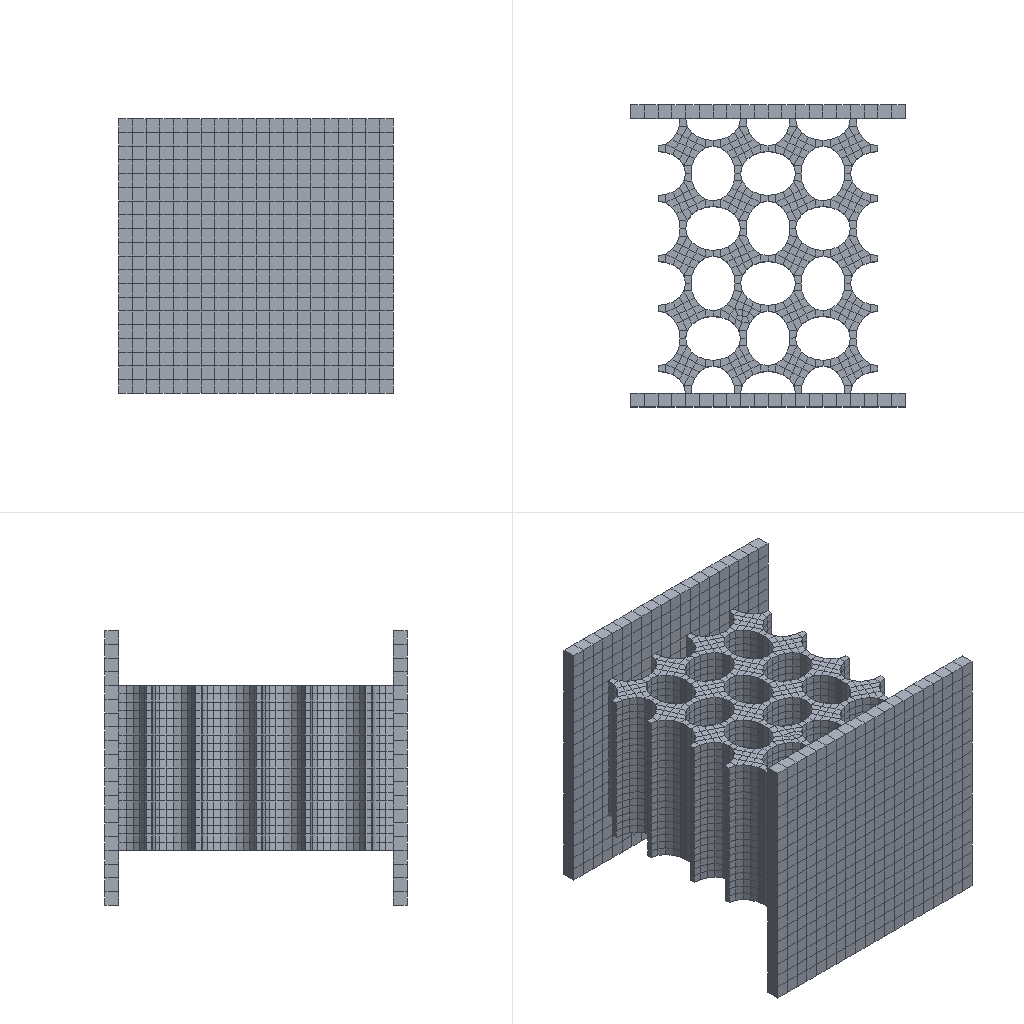Simulation study | abaqus
Set-up summary:
category,name,step,type,value,unit,region
solver,abaqus,,Abaqus/CAE 2024
units,mm-N-s-tonne (MPa),,inferred,E=210000 density=7.89e-09
analysis,Step-1,,dynamic explicit,nlgeom=True; time_period=0.1
mesh,nodes,,,14387
mesh,elements,,,8860
element_type,C3D8R,,,8860
material,Steel,,E,210000
material,Steel,,nu,0.3
material,Steel,,density,7.89e-09
material,TPU,,E,450
material,TPU,,nu,0.38
material,TPU,,density,1.25e-09
material,TPU,,yield,28
material,TPU,,behaviors,plastic
section,Steel,,solid section,,,Bottom
section,Steel,,solid section,,,Head
section,TPU,,solid section,,,JG
bc,BC-1,initial,encastre,[dofs=ENCASTRE],,_PickedSet27
bc,BC-2,Step-1,fixed,"[dofs=rx,ry,rz,x,z n=5]",,_PickedSet28
bc,BC-2,Step-1,displacement,-10 [dofs=y],,_PickedSet28
contact,Int-1,initial,general contact,interaction=IntProp-1; friction=0.2; behavior=hard
constraint,rigid body,,,2
Abaqus input file, long lists of numbers shortened:
*Heading
** Job name: deck Model name: 0204
** Generated by: Abaqus/CAE 2024
*Preprint, echo=NO, model=NO, history=NO, contact=NO
**
** PARTS
**
*Part, name=Bottom
*Node
      1,          20.,          20.,           1.
      2,          20.,          19.,           1.
** (880 more lines like these left out)
*Element, type=C3D8R
  1,  43,  44,  65,  64,   1,   2,  23,  22
  2,  44,  45,  66,  65,   2,   3,  24,  23
** (398 more lines like these left out)
*Nset, nset=Bottom, generate
   1,  882,    1
*Elset, elset=Bottom, generate
   1,  400,    1
** Section: YABAN
*Solid Section, elset=Bottom, material=Steel
,
*End Part
**
*Part, name=Head
*Node
      1,          20.,          20.,           1.
      2,          20.,          19.,           1.
** (880 more lines like these left out)
*Element, type=C3D8R
  1,  43,  44,  65,  64,   1,   2,  23,  22
  2,  44,  45,  66,  65,   2,   3,  24,  23
** (398 more lines like these left out)
*Nset, nset=Head, generate
   1,  882,    1
*Elset, elset=Head, generate
   1,  400,    1
** Section: YABAN
*Solid Section, elset=Head, material=Steel
,
*End Part
**
*Part, name=JG
*Node
      1,    11.453,   17.88,           0.
      2,   10.995,   17.556,           0.
** (12619 more lines like these left out)
*Element, type=C3D8R
   1,    15,   222,   221,    16,   616,   823,   822,   617
   2,    15,   419,   393,   222,   616,  1020,   994,   823
** (8058 more lines like these left out)
*Nset, nset=JG, generate
     1,  12621,      1
*Elset, elset=JG, generate
    1,  8060,     1
** Section: JG
*Solid Section, elset=JG, material=TPU
,
*End Part
**
**
** ASSEMBLY
**
*Assembly, name=Assembly
**
*Instance, name=Bottom-1, part=Bottom
        39.6,          -1.,          12.
        39.6,          -1.,          12., 38.6,          -1.,          12., 90.
*End Instance
**
*Instance, name=Head-1, part=Head
        39.6,          20.,          12.
        39.6,          20.,          12., 38.6,          20.,          12., 90.
*End Instance
**
*Instance, name=JG-1, part=JG
        41.6,           0.,          -4.
*End Instance
**
*Node
      1,   49.6,          21.,           2.
*Node
      2,   49.6,          -1.,           2.
*Nset, nset=rp
 1,
*Nset, nset=_PickedSet14, internal, instance=Bottom-1, generate
   1,  882,    1
*Elset, elset=_PickedSet14, internal, instance=Bottom-1, generate
   1,  400,    1
*Nset, nset=_PickedSet16, internal, instance=Head-1, generate
   1,  882,    1
*Elset, elset=_PickedSet16, internal, instance=Head-1, generate
   1,  400,    1
*Nset, nset=_PickedSet25, internal
 2,
*Nset, nset=_PickedSet26, internal
 1,
*Nset, nset=_PickedSet27, internal
 2,
*Nset, nset=_PickedSet28, internal
 1,
*Elset, elset=_D_S3, internal, instance=Bottom-1, generate
   1,  400,    1
*Surface, type=ELEMENT, name=D
_D_S3, S3
*Elset, elset=_D1_S3, internal, instance=JG-1
  213,  219,  616,  622, 1019, 1025, 1422, 1428, 1825, 1831, 2228, 2234, 2631, 2637, 3034, 3040
 3437, 3443, 3840, 3846, 4243, 4249, 4646, 4652, 5049, 5055, 5452, 5458, 5855, 5861, 6258, 6264
** (1 more lines like these left out)
*Elset, elset=_D1_S4, internal, instance=JG-1
   80,  223,  483,  626,  886, 1029, 1289, 1432, 1692, 1835, 2095, 2238, 2498, 2641, 2901, 3044
 3304, 3447, 3707, 3850, 4110, 4253, 4513, 4656, 4916, 5059, 5319, 5462, 5722, 5865, 6125, 6268
** (1 more lines like these left out)
*Surface, type=ELEMENT, name=D1
_D1_S3, S3
_D1_S4, S4
*Elset, elset=_U_S5, internal, instance=Head-1, generate
   1,  400,    1
*Surface, type=ELEMENT, name=U
_U_S5, S5
*Elset, elset=_U1_S4, internal, instance=JG-1
  186,  195,  589,  598,  992, 1001, 1395, 1404, 1798, 1807, 2201, 2210, 2604, 2613, 3007, 3016
 3410, 3419, 3813, 3822, 4216, 4225, 4619, 4628, 5022, 5031, 5425, 5434, 5828, 5837, 6231, 6240
** (1 more lines like these left out)
*Elset, elset=_U1_S5, internal, instance=JG-1
  191,  201,  594,  604,  997, 1007, 1400, 1410, 1803, 1813, 2206, 2216, 2609, 2619, 3012, 3022
 3415, 3425, 3818, 3828, 4221, 4231, 4624, 4634, 5027, 5037, 5430, 5440, 5833, 5843, 6236, 6246
** (1 more lines like these left out)
*Surface, type=ELEMENT, name=U1
_U1_S4, S4
_U1_S5, S5
** Constraint: Constraint-1
*Rigid Body, ref node=_PickedSet25, elset=_PickedSet14
** Constraint: Constraint-2
*Rigid Body, ref node=_PickedSet26, elset=_PickedSet16
*End Assembly
*Amplitude, name=Amp-1
             0.,              0.,             0.1,              1.
**
** MATERIALS
**
*Material, name=Steel
*Density
 7.89e-09,
*Elastic
210000., 0.3
*Material, name=TPU
*Density
 1.25e-09,
*Elastic
450., 0.38
*Plastic
28.,   0.
35., 0.05
42., 0.15
50.,  0.3
60.,  0.6
75.,   1.
**
** INTERACTION PROPERTIES
**
*Surface Interaction, name=IntProp-1
*Friction
 0.2,
*Surface Behavior, pressure-overclosure=HARD
**
** BOUNDARY CONDITIONS
**
** Name: BC-1 Type: Symmetry/Antisymmetry/Encastre
*Boundary
_PickedSet27, ENCASTRE
**
** INTERACTIONS
**
** Interaction: Int-1
*Contact, op=NEW
*Contact Inclusions, ALL EXTERIOR
*Contact Property Assignment
 ,  , IntProp-1
** ----------------------------------------------------------------
**
** STEP: Step-1
**
*Step, name=Step-1, nlgeom=YES
*Dynamic, Explicit
, 0.1
*Bulk Viscosity
0.06, 1.2
** Mass Scaling: Semi-Automatic
**               Whole Model
*Fixed Mass Scaling, factor=100.
**
** BOUNDARY CONDITIONS
**
** Name: BC-2 Type: Displacement/Rotation
*Boundary, amplitude=Amp-1
_PickedSet28, 1, 1
_PickedSet28, 2, 2, -10.
_PickedSet28, 3, 3
_PickedSet28, 4, 4
_PickedSet28, 5, 5
_PickedSet28, 6, 6
**
** OUTPUT REQUESTS
**
*Restart, write, number interval=1, time marks=NO
**
** FIELD OUTPUT: F-Output-1
**
*Output, field
*Node Output
RF, U, V
*Element Output, directions=YES
E, LE, MISES, PE, PEEQ, PEMAG, S
**
** HISTORY OUTPUT: H-Output-2
**
*Output, history, frequency=1
*Node Output, nset=rp
RF1, RF2, RF3, U1, U2, U3
**
** HISTORY OUTPUT: H-Output-1
**
*Output, history, variable=PRESELECT, frequency=1
*End Step
Results summary:
result,odb.job_status,,,JOB_STATUS_COMPLETED_SUCCESSFULLY,"consistent, unstated (Abaqus has no unit system)"
result,steps[0].procedure,Step-1,,"*DYNAMIC, EXPLICIT","consistent, unstated (Abaqus has no unit system)"
result,steps[0].time_period,Step-1,,0.1,"consistent, unstated (Abaqus has no unit system)"
result,steps[0].n_frames,Step-1,,21,"consistent, unstated (Abaqus has no unit system)"
result,steps[0].last_frame.id,Step-1,,24140,"consistent, unstated (Abaqus has no unit system)"
result,steps[0].last_frame.value,Step-1,,0.1,"consistent, unstated (Abaqus has no unit system)"
result,steps[0].last_frame.description,Step-1,,Increment     24140: Step Time =   0.1,"consistent, unstated (Abaqus has no unit system)"
result,steps[0].completed,Step-1,,True,"consistent, unstated (Abaqus has no unit system)"
result,steps[0].max_U_magnitude,Step-1,,10.482,"consistent, unstated (Abaqus has no unit system)"
result,steps[0].max_S_mises,Step-1,,49.03,"consistent, unstated (Abaqus has no unit system)"
result,steps[0].RF_sum[1],Step-1,,9.59,"consistent, unstated (Abaqus has no unit system)"
result,steps[0].RF_sum[2],Step-1,,-3.462,"consistent, unstated (Abaqus has no unit system)"
result,steps[0].RF_sum[3],Step-1,,0.1568,"consistent, unstated (Abaqus has no unit system)"
result,steps[0].diagnostic.n_increments,Step-1,,21,"consistent, unstated (Abaqus has no unit system)"